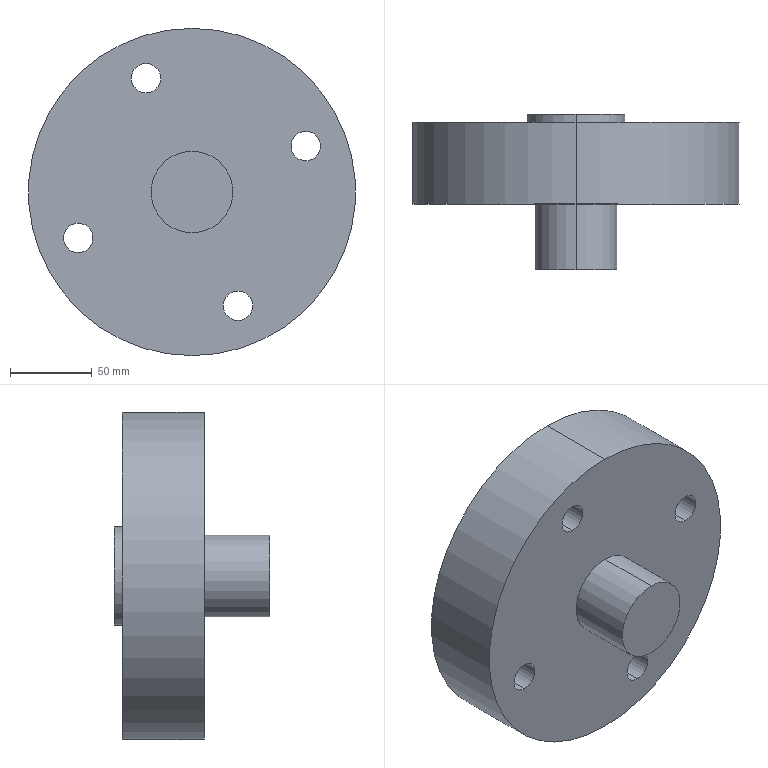Part | SolidWorks | features Chamfer 1, HoleWzd 1, Revolution 1 | 1 solid | 18 faces | box 200 x 95 x 200 mm | volume 1612580 mm3 | cylinder 14 | plane 4 | commonest cylinder face diameters 18 x8 50 x2 60 x2 200 x2
STEP:
#1=CARTESIAN_POINT('',(-69.533,-81.6,-19.109));
#2=VERTEX_POINT('',#1);
#3=CARTESIAN_POINT('',(-69.533,-81.6,-37.109));
#4=VERTEX_POINT('',#3);
#5=CARTESIAN_POINT('',(-69.533,-81.6,-28.109));
#6=DIRECTION('',(0.,-1.,0.));
#7=DIRECTION('',(0.,0.,-1.));
#8=AXIS2_PLACEMENT_3D('',#5,#6,#7);
#9=CIRCLE('',#8,9.);
#10=EDGE_CURVE('',#2,#4,#9,.T.);
#11=ORIENTED_EDGE('',*,*,#10,.T.);
#12=CARTESIAN_POINT('',(-69.533,-31.6,-37.109));
#13=VERTEX_POINT('',#12);
#14=CARTESIAN_POINT('',(-69.533,-31.6,-37.109));
#15=DIRECTION('',(0.,1.,0.));
#16=VECTOR('',#15,1000.);
#17=LINE('',#14,#16);
#18=EDGE_CURVE('',#4,#13,#17,.T.);
#19=ORIENTED_EDGE('',*,*,#18,.T.);
#20=CARTESIAN_POINT('',(-69.533,-31.6,-19.109));
#21=VERTEX_POINT('',#20);
#22=CARTESIAN_POINT('',(-69.533,-31.6,-28.109));
#23=DIRECTION('',(0.,1.,0.));
#24=DIRECTION('',(0.,0.,1.));
#25=AXIS2_PLACEMENT_3D('',#22,#23,#24);
#26=CIRCLE('',#25,9.);
#27=EDGE_CURVE('',#13,#21,#26,.T.);
#28=ORIENTED_EDGE('',*,*,#27,.T.);
#29=CARTESIAN_POINT('',(-69.533,-31.6,-19.109));
#30=DIRECTION('',(0.,1.,0.));
#31=VECTOR('',#30,1000.);
#32=LINE('',#29,#31);
#33=EDGE_CURVE('',#2,#21,#32,.T.);
#34=ORIENTED_EDGE('',*,*,#33,.F.);
#35=EDGE_LOOP('',(#11,#19,#28,#34));
#36=FACE_OUTER_BOUND('',#35,.T.);
#37=CARTESIAN_POINT('',(-69.533,-31.6,-28.109));
#38=DIRECTION('',(0.,1.,0.));
#39=DIRECTION('',(0.,0.,1.));
#40=AXIS2_PLACEMENT_3D('',#37,#38,#39);
#41=CYLINDRICAL_SURFACE('',#40,9.);
#42=ADVANCED_FACE('',(#36),#41,.F.);
#43=CARTESIAN_POINT('',(-28.109,-81.6,78.533));
#44=VERTEX_POINT('',#43);
#45=CARTESIAN_POINT('',(-28.109,-81.6,60.533));
#46=VERTEX_POINT('',#45);
#47=CARTESIAN_POINT('',(-28.109,-81.6,69.533));
#48=DIRECTION('',(0.,-1.,0.));
#49=DIRECTION('',(0.,0.,-1.));
#50=AXIS2_PLACEMENT_3D('',#47,#48,#49);
#51=CIRCLE('',#50,9.);
#52=EDGE_CURVE('',#44,#46,#51,.T.);
#53=ORIENTED_EDGE('',*,*,#52,.T.);
#54=CARTESIAN_POINT('',(-28.109,-31.6,60.533));
#55=VERTEX_POINT('',#54);
#56=CARTESIAN_POINT('',(-28.109,-31.6,60.533));
#57=DIRECTION('',(0.,1.,0.));
#58=VECTOR('',#57,1000.);
#59=LINE('',#56,#58);
#60=EDGE_CURVE('',#46,#55,#59,.T.);
#61=ORIENTED_EDGE('',*,*,#60,.T.);
#62=CARTESIAN_POINT('',(-28.109,-31.6,78.533));
#63=VERTEX_POINT('',#62);
#64=CARTESIAN_POINT('',(-28.109,-31.6,69.533));
#65=DIRECTION('',(0.,1.,0.));
#66=DIRECTION('',(0.,0.,1.));
#67=AXIS2_PLACEMENT_3D('',#64,#65,#66);
#68=CIRCLE('',#67,9.);
#69=EDGE_CURVE('',#55,#63,#68,.T.);
#70=ORIENTED_EDGE('',*,*,#69,.T.);
#71=CARTESIAN_POINT('',(-28.109,-31.6,78.533));
#72=DIRECTION('',(0.,1.,0.));
#73=VECTOR('',#72,1000.);
#74=LINE('',#71,#73);
#75=EDGE_CURVE('',#44,#63,#74,.T.);
#76=ORIENTED_EDGE('',*,*,#75,.F.);
#77=EDGE_LOOP('',(#53,#61,#70,#76));
#78=FACE_OUTER_BOUND('',#77,.T.);
#79=CARTESIAN_POINT('',(-28.109,-31.6,69.533));
#80=DIRECTION('',(0.,1.,0.));
#81=DIRECTION('',(0.,0.,1.));
#82=AXIS2_PLACEMENT_3D('',#79,#80,#81);
#83=CYLINDRICAL_SURFACE('',#82,9.);
#84=ADVANCED_FACE('',(#78),#83,.F.);
#85=CARTESIAN_POINT('',(69.533,-81.6,37.109));
#86=VERTEX_POINT('',#85);
#87=CARTESIAN_POINT('',(69.533,-81.6,19.109));
#88=VERTEX_POINT('',#87);
#89=CARTESIAN_POINT('',(69.533,-81.6,28.109));
#90=DIRECTION('',(0.,-1.,0.));
#91=DIRECTION('',(0.,0.,-1.));
#92=AXIS2_PLACEMENT_3D('',#89,#90,#91);
#93=CIRCLE('',#92,9.);
#94=EDGE_CURVE('',#86,#88,#93,.T.);
#95=ORIENTED_EDGE('',*,*,#94,.T.);
#96=CARTESIAN_POINT('',(69.533,-31.6,19.109));
#97=VERTEX_POINT('',#96);
#98=CARTESIAN_POINT('',(69.533,-31.6,19.109));
#99=DIRECTION('',(0.,1.,0.));
#100=VECTOR('',#99,1000.);
#101=LINE('',#98,#100);
#102=EDGE_CURVE('',#88,#97,#101,.T.);
#103=ORIENTED_EDGE('',*,*,#102,.T.);
#104=CARTESIAN_POINT('',(69.533,-31.6,37.109));
#105=VERTEX_POINT('',#104);
#106=CARTESIAN_POINT('',(69.533,-31.6,28.109));
#107=DIRECTION('',(0.,1.,0.));
#108=DIRECTION('',(0.,0.,1.));
#109=AXIS2_PLACEMENT_3D('',#106,#107,#108);
#110=CIRCLE('',#109,9.);
#111=EDGE_CURVE('',#97,#105,#110,.T.);
#112=ORIENTED_EDGE('',*,*,#111,.T.);
#113=CARTESIAN_POINT('',(69.533,-31.6,37.109));
#114=DIRECTION('',(0.,1.,0.));
#115=VECTOR('',#114,1000.);
#116=LINE('',#113,#115);
#117=EDGE_CURVE('',#86,#105,#116,.T.);
#118=ORIENTED_EDGE('',*,*,#117,.F.);
#119=EDGE_LOOP('',(#95,#103,#112,#118));
#120=FACE_OUTER_BOUND('',#119,.T.);
#121=CARTESIAN_POINT('',(69.533,-31.6,28.109));
#122=DIRECTION('',(0.,1.,0.));
#123=DIRECTION('',(0.,0.,1.));
#124=AXIS2_PLACEMENT_3D('',#121,#122,#123);
#125=CYLINDRICAL_SURFACE('',#124,9.);
#126=ADVANCED_FACE('',(#120),#125,.F.);
#127=CARTESIAN_POINT('',(28.109,-81.6,-60.533));
#128=VERTEX_POINT('',#127);
#129=CARTESIAN_POINT('',(28.109,-81.6,-78.533));
#130=VERTEX_POINT('',#129);
#131=CARTESIAN_POINT('',(28.109,-81.6,-69.533));
#132=DIRECTION('',(0.,-1.,0.));
#133=DIRECTION('',(0.,0.,-1.));
#134=AXIS2_PLACEMENT_3D('',#131,#132,#133);
#135=CIRCLE('',#134,9.);
#136=EDGE_CURVE('',#128,#130,#135,.T.);
#137=ORIENTED_EDGE('',*,*,#136,.T.);
#138=CARTESIAN_POINT('',(28.109,-31.6,-78.533));
#139=VERTEX_POINT('',#138);
#140=CARTESIAN_POINT('',(28.109,-31.6,-78.533));
#141=DIRECTION('',(0.,1.,0.));
#142=VECTOR('',#141,1000.);
#143=LINE('',#140,#142);
#144=EDGE_CURVE('',#130,#139,#143,.T.);
#145=ORIENTED_EDGE('',*,*,#144,.T.);
#146=CARTESIAN_POINT('',(28.109,-31.6,-60.533));
#147=VERTEX_POINT('',#146);
#148=CARTESIAN_POINT('',(28.109,-31.6,-69.533));
#149=DIRECTION('',(0.,1.,0.));
#150=DIRECTION('',(0.,0.,1.));
#151=AXIS2_PLACEMENT_3D('',#148,#149,#150);
#152=CIRCLE('',#151,9.);
#153=EDGE_CURVE('',#139,#147,#152,.T.);
#154=ORIENTED_EDGE('',*,*,#153,.T.);
#155=CARTESIAN_POINT('',(28.109,-31.6,-60.533));
#156=DIRECTION('',(0.,1.,0.));
#157=VECTOR('',#156,1000.);
#158=LINE('',#155,#157);
#159=EDGE_CURVE('',#128,#147,#158,.T.);
#160=ORIENTED_EDGE('',*,*,#159,.F.);
#161=EDGE_LOOP('',(#137,#145,#154,#160));
#162=FACE_OUTER_BOUND('',#161,.T.);
#163=CARTESIAN_POINT('',(28.109,-31.6,-69.533));
#164=DIRECTION('',(0.,1.,0.));
#165=DIRECTION('',(0.,0.,1.));
#166=AXIS2_PLACEMENT_3D('',#163,#164,#165);
#167=CYLINDRICAL_SURFACE('',#166,9.);
#168=ADVANCED_FACE('',(#162),#167,.F.);
#169=CARTESIAN_POINT('',(0.,-26.6,-30.));
#170=VERTEX_POINT('',#169);
#171=CARTESIAN_POINT('',(0.,-26.6,30.));
#172=VERTEX_POINT('',#171);
#173=CARTESIAN_POINT('',(0.,-26.6,0.));
#174=DIRECTION('',(0.,-1.,0.));
#175=DIRECTION('',(0.,0.,-1.));
#176=AXIS2_PLACEMENT_3D('',#173,#174,#175);
#177=CIRCLE('',#176,30.);
#178=EDGE_CURVE('',#170,#172,#177,.T.);
#179=ORIENTED_EDGE('',*,*,#178,.T.);
#180=CARTESIAN_POINT('',(0.,-31.6,30.));
#181=VERTEX_POINT('',#180);
#182=CARTESIAN_POINT('',(0.,0.,30.));
#183=DIRECTION('',(0.,-1.,0.));
#184=VECTOR('',#183,1000.);
#185=LINE('',#182,#184);
#186=EDGE_CURVE('',#172,#181,#185,.T.);
#187=ORIENTED_EDGE('',*,*,#186,.T.);
#188=CARTESIAN_POINT('',(0.,-31.6,-30.));
#189=VERTEX_POINT('',#188);
#190=CARTESIAN_POINT('',(0.,-31.6,0.));
#191=DIRECTION('',(0.,-1.,0.));
#192=DIRECTION('',(0.,0.,-1.));
#193=AXIS2_PLACEMENT_3D('',#190,#191,#192);
#194=CIRCLE('',#193,30.);
#195=EDGE_CURVE('',#189,#181,#194,.T.);
#196=ORIENTED_EDGE('',*,*,#195,.F.);
#197=CARTESIAN_POINT('',(0.,0.,-30.));
#198=DIRECTION('',(0.,-1.,0.));
#199=VECTOR('',#198,1000.);
#200=LINE('',#197,#199);
#201=EDGE_CURVE('',#170,#189,#200,.T.);
#202=ORIENTED_EDGE('',*,*,#201,.F.);
#203=EDGE_LOOP('',(#179,#187,#196,#202));
#204=FACE_OUTER_BOUND('',#203,.T.);
#205=CARTESIAN_POINT('',(0.,0.,0.));
#206=DIRECTION('',(0.,-1.,0.));
#207=DIRECTION('',(0.,0.,-1.));
#208=AXIS2_PLACEMENT_3D('',#205,#206,#207);
#209=CYLINDRICAL_SURFACE('',#208,30.);
#210=ADVANCED_FACE('',(#204),#209,.T.);
#211=CARTESIAN_POINT('',(0.,-31.6,-100.));
#212=VERTEX_POINT('',#211);
#213=CARTESIAN_POINT('',(0.,-31.6,100.));
#214=VERTEX_POINT('',#213);
#215=CARTESIAN_POINT('',(0.,-31.6,0.));
#216=DIRECTION('',(0.,-1.,0.));
#217=DIRECTION('',(0.,0.,-1.));
#218=AXIS2_PLACEMENT_3D('',#215,#216,#217);
#219=CIRCLE('',#218,100.);
#220=EDGE_CURVE('',#212,#214,#219,.T.);
#221=ORIENTED_EDGE('',*,*,#220,.T.);
#222=CARTESIAN_POINT('',(0.,-81.6,100.));
#223=VERTEX_POINT('',#222);
#224=CARTESIAN_POINT('',(0.,0.,100.));
#225=DIRECTION('',(0.,-1.,0.));
#226=VECTOR('',#225,1000.);
#227=LINE('',#224,#226);
#228=EDGE_CURVE('',#214,#223,#227,.T.);
#229=ORIENTED_EDGE('',*,*,#228,.T.);
#230=CARTESIAN_POINT('',(0.,-81.6,-100.));
#231=VERTEX_POINT('',#230);
#232=CARTESIAN_POINT('',(0.,-81.6,0.));
#233=DIRECTION('',(0.,-1.,0.));
#234=DIRECTION('',(0.,0.,-1.));
#235=AXIS2_PLACEMENT_3D('',#232,#233,#234);
#236=CIRCLE('',#235,100.);
#237=EDGE_CURVE('',#231,#223,#236,.T.);
#238=ORIENTED_EDGE('',*,*,#237,.F.);
#239=CARTESIAN_POINT('',(0.,0.,-100.));
#240=DIRECTION('',(0.,-1.,0.));
#241=VECTOR('',#240,1000.);
#242=LINE('',#239,#241);
#243=EDGE_CURVE('',#212,#231,#242,.T.);
#244=ORIENTED_EDGE('',*,*,#243,.F.);
#245=EDGE_LOOP('',(#221,#229,#238,#244));
#246=FACE_OUTER_BOUND('',#245,.T.);
#247=CARTESIAN_POINT('',(0.,0.,0.));
#248=DIRECTION('',(0.,-1.,0.));
#249=DIRECTION('',(0.,0.,-1.));
#250=AXIS2_PLACEMENT_3D('',#247,#248,#249);
#251=CYLINDRICAL_SURFACE('',#250,100.);
#252=ADVANCED_FACE('',(#246),#251,.T.);
#253=CARTESIAN_POINT('',(0.,-81.6,-25.));
#254=VERTEX_POINT('',#253);
#255=CARTESIAN_POINT('',(0.,-81.6,25.));
#256=VERTEX_POINT('',#255);
#257=CARTESIAN_POINT('',(0.,-81.6,0.));
#258=DIRECTION('',(0.,-1.,0.));
#259=DIRECTION('',(0.,0.,-1.));
#260=AXIS2_PLACEMENT_3D('',#257,#258,#259);
#261=CIRCLE('',#260,25.);
#262=EDGE_CURVE('',#254,#256,#261,.T.);
#263=ORIENTED_EDGE('',*,*,#262,.T.);
#264=CARTESIAN_POINT('',(0.,-121.6,25.));
#265=VERTEX_POINT('',#264);
#266=CARTESIAN_POINT('',(0.,0.,25.));
#267=DIRECTION('',(0.,-1.,0.));
#268=VECTOR('',#267,1000.);
#269=LINE('',#266,#268);
#270=EDGE_CURVE('',#256,#265,#269,.T.);
#271=ORIENTED_EDGE('',*,*,#270,.T.);
#272=CARTESIAN_POINT('',(0.,-121.6,-25.));
#273=VERTEX_POINT('',#272);
#274=CARTESIAN_POINT('',(0.,-121.6,0.));
#275=DIRECTION('',(0.,-1.,0.));
#276=DIRECTION('',(0.,0.,-1.));
#277=AXIS2_PLACEMENT_3D('',#274,#275,#276);
#278=CIRCLE('',#277,25.);
#279=EDGE_CURVE('',#273,#265,#278,.T.);
#280=ORIENTED_EDGE('',*,*,#279,.F.);
#281=CARTESIAN_POINT('',(0.,0.,-25.));
#282=DIRECTION('',(0.,-1.,0.));
#283=VECTOR('',#282,1000.);
#284=LINE('',#281,#283);
#285=EDGE_CURVE('',#254,#273,#284,.T.);
#286=ORIENTED_EDGE('',*,*,#285,.F.);
#287=EDGE_LOOP('',(#263,#271,#280,#286));
#288=FACE_OUTER_BOUND('',#287,.T.);
#289=CARTESIAN_POINT('',(0.,0.,0.));
#290=DIRECTION('',(0.,-1.,0.));
#291=DIRECTION('',(0.,0.,-1.));
#292=AXIS2_PLACEMENT_3D('',#289,#290,#291);
#293=CYLINDRICAL_SURFACE('',#292,25.);
#294=ADVANCED_FACE('',(#288),#293,.T.);
#295=ORIENTED_EDGE('',*,*,#279,.T.);
#296=CARTESIAN_POINT('',(0.,-121.6,0.));
#297=DIRECTION('',(0.,-1.,0.));
#298=DIRECTION('',(0.,0.,-1.));
#299=AXIS2_PLACEMENT_3D('',#296,#297,#298);
#300=CIRCLE('',#299,25.);
#301=EDGE_CURVE('',#265,#273,#300,.T.);
#302=ORIENTED_EDGE('',*,*,#301,.T.);
#303=EDGE_LOOP('',(#295,#302));
#304=FACE_OUTER_BOUND('',#303,.T.);
#305=CARTESIAN_POINT('',(25.,-121.6,0.));
#306=DIRECTION('',(0.,-1.,0.));
#307=DIRECTION('',(0.,0.,-1.));
#308=AXIS2_PLACEMENT_3D('',#305,#306,#307);
#309=PLANE('',#308);
#310=ADVANCED_FACE('',(#304),#309,.T.);
#311=ORIENTED_EDGE('',*,*,#270,.F.);
#312=CARTESIAN_POINT('',(0.,-81.6,0.));
#313=DIRECTION('',(0.,-1.,0.));
#314=DIRECTION('',(0.,0.,-1.));
#315=AXIS2_PLACEMENT_3D('',#312,#313,#314);
#316=CIRCLE('',#315,25.);
#317=EDGE_CURVE('',#256,#254,#316,.T.);
#318=ORIENTED_EDGE('',*,*,#317,.T.);
#319=ORIENTED_EDGE('',*,*,#285,.T.);
#320=ORIENTED_EDGE('',*,*,#301,.F.);
#321=EDGE_LOOP('',(#311,#318,#319,#320));
#322=FACE_OUTER_BOUND('',#321,.T.);
#323=CARTESIAN_POINT('',(0.,0.,0.));
#324=DIRECTION('',(0.,-1.,0.));
#325=DIRECTION('',(0.,0.,-1.));
#326=AXIS2_PLACEMENT_3D('',#323,#324,#325);
#327=CYLINDRICAL_SURFACE('',#326,25.);
#328=ADVANCED_FACE('',(#322),#327,.T.);
#329=ORIENTED_EDGE('',*,*,#10,.F.);
#330=CARTESIAN_POINT('',(-69.533,-81.6,-28.109));
#331=DIRECTION('',(0.,-1.,0.));
#332=DIRECTION('',(0.,0.,-1.));
#333=AXIS2_PLACEMENT_3D('',#330,#331,#332);
#334=CIRCLE('',#333,9.);
#335=EDGE_CURVE('',#4,#2,#334,.T.);
#336=ORIENTED_EDGE('',*,*,#335,.F.);
#337=EDGE_LOOP('',(#329,#336));
#338=FACE_BOUND('',#337,.T.);
#339=ORIENTED_EDGE('',*,*,#52,.F.);
#340=CARTESIAN_POINT('',(-28.109,-81.6,69.533));
#341=DIRECTION('',(0.,-1.,0.));
#342=DIRECTION('',(0.,0.,-1.));
#343=AXIS2_PLACEMENT_3D('',#340,#341,#342);
#344=CIRCLE('',#343,9.);
#345=EDGE_CURVE('',#46,#44,#344,.T.);
#346=ORIENTED_EDGE('',*,*,#345,.F.);
#347=EDGE_LOOP('',(#339,#346));
#348=FACE_BOUND('',#347,.T.);
#349=ORIENTED_EDGE('',*,*,#94,.F.);
#350=CARTESIAN_POINT('',(69.533,-81.6,28.109));
#351=DIRECTION('',(0.,-1.,0.));
#352=DIRECTION('',(0.,0.,-1.));
#353=AXIS2_PLACEMENT_3D('',#350,#351,#352);
#354=CIRCLE('',#353,9.);
#355=EDGE_CURVE('',#88,#86,#354,.T.);
#356=ORIENTED_EDGE('',*,*,#355,.F.);
#357=EDGE_LOOP('',(#349,#356));
#358=FACE_BOUND('',#357,.T.);
#359=ORIENTED_EDGE('',*,*,#136,.F.);
#360=CARTESIAN_POINT('',(28.109,-81.6,-69.533));
#361=DIRECTION('',(0.,-1.,0.));
#362=DIRECTION('',(0.,0.,-1.));
#363=AXIS2_PLACEMENT_3D('',#360,#361,#362);
#364=CIRCLE('',#363,9.);
#365=EDGE_CURVE('',#130,#128,#364,.T.);
#366=ORIENTED_EDGE('',*,*,#365,.F.);
#367=EDGE_LOOP('',(#359,#366));
#368=FACE_BOUND('',#367,.T.);
#369=ORIENTED_EDGE('',*,*,#237,.T.);
#370=CARTESIAN_POINT('',(0.,-81.6,0.));
#371=DIRECTION('',(0.,-1.,0.));
#372=DIRECTION('',(0.,0.,-1.));
#373=AXIS2_PLACEMENT_3D('',#370,#371,#372);
#374=CIRCLE('',#373,100.);
#375=EDGE_CURVE('',#223,#231,#374,.T.);
#376=ORIENTED_EDGE('',*,*,#375,.T.);
#377=EDGE_LOOP('',(#369,#376));
#378=FACE_OUTER_BOUND('',#377,.T.);
#379=ORIENTED_EDGE('',*,*,#262,.F.);
#380=ORIENTED_EDGE('',*,*,#317,.F.);
#381=EDGE_LOOP('',(#379,#380));
#382=FACE_BOUND('',#381,.T.);
#383=CARTESIAN_POINT('',(100.,-81.6,0.));
#384=DIRECTION('',(0.,-1.,0.));
#385=DIRECTION('',(0.,0.,-1.));
#386=AXIS2_PLACEMENT_3D('',#383,#384,#385);
#387=PLANE('',#386);
#388=ADVANCED_FACE('',(#338,#348,#358,#368,#378,#382),#387,.T.);
#389=ORIENTED_EDGE('',*,*,#228,.F.);
#390=CARTESIAN_POINT('',(0.,-31.6,0.));
#391=DIRECTION('',(0.,-1.,0.));
#392=DIRECTION('',(0.,0.,-1.));
#393=AXIS2_PLACEMENT_3D('',#390,#391,#392);
#394=CIRCLE('',#393,100.);
#395=EDGE_CURVE('',#214,#212,#394,.T.);
#396=ORIENTED_EDGE('',*,*,#395,.T.);
#397=ORIENTED_EDGE('',*,*,#243,.T.);
#398=ORIENTED_EDGE('',*,*,#375,.F.);
#399=EDGE_LOOP('',(#389,#396,#397,#398));
#400=FACE_OUTER_BOUND('',#399,.T.);
#401=CARTESIAN_POINT('',(0.,0.,0.));
#402=DIRECTION('',(0.,-1.,0.));
#403=DIRECTION('',(0.,0.,-1.));
#404=AXIS2_PLACEMENT_3D('',#401,#402,#403);
#405=CYLINDRICAL_SURFACE('',#404,100.);
#406=ADVANCED_FACE('',(#400),#405,.T.);
#407=CARTESIAN_POINT('',(-69.533,-31.6,-28.109));
#408=DIRECTION('',(0.,1.,0.));
#409=DIRECTION('',(0.,0.,1.));
#410=AXIS2_PLACEMENT_3D('',#407,#408,#409);
#411=CIRCLE('',#410,9.);
#412=EDGE_CURVE('',#21,#13,#411,.T.);
#413=ORIENTED_EDGE('',*,*,#412,.F.);
#414=ORIENTED_EDGE('',*,*,#27,.F.);
#415=EDGE_LOOP('',(#413,#414));
#416=FACE_BOUND('',#415,.T.);
#417=CARTESIAN_POINT('',(-28.109,-31.6,69.533));
#418=DIRECTION('',(0.,1.,0.));
#419=DIRECTION('',(0.,0.,1.));
#420=AXIS2_PLACEMENT_3D('',#417,#418,#419);
#421=CIRCLE('',#420,9.);
#422=EDGE_CURVE('',#63,#55,#421,.T.);
#423=ORIENTED_EDGE('',*,*,#422,.F.);
#424=ORIENTED_EDGE('',*,*,#69,.F.);
#425=EDGE_LOOP('',(#423,#424));
#426=FACE_BOUND('',#425,.T.);
#427=CARTESIAN_POINT('',(69.533,-31.6,28.109));
#428=DIRECTION('',(0.,1.,0.));
#429=DIRECTION('',(0.,0.,1.));
#430=AXIS2_PLACEMENT_3D('',#427,#428,#429);
#431=CIRCLE('',#430,9.);
#432=EDGE_CURVE('',#105,#97,#431,.T.);
#433=ORIENTED_EDGE('',*,*,#432,.F.);
#434=ORIENTED_EDGE('',*,*,#111,.F.);
#435=EDGE_LOOP('',(#433,#434));
#436=FACE_BOUND('',#435,.T.);
#437=CARTESIAN_POINT('',(28.109,-31.6,-69.533));
#438=DIRECTION('',(0.,1.,0.));
#439=DIRECTION('',(0.,0.,1.));
#440=AXIS2_PLACEMENT_3D('',#437,#438,#439);
#441=CIRCLE('',#440,9.);
#442=EDGE_CURVE('',#147,#139,#441,.T.);
#443=ORIENTED_EDGE('',*,*,#442,.F.);
#444=ORIENTED_EDGE('',*,*,#153,.F.);
#445=EDGE_LOOP('',(#443,#444));
#446=FACE_BOUND('',#445,.T.);
#447=ORIENTED_EDGE('',*,*,#195,.T.);
#448=CARTESIAN_POINT('',(0.,-31.6,0.));
#449=DIRECTION('',(0.,-1.,0.));
#450=DIRECTION('',(0.,0.,-1.));
#451=AXIS2_PLACEMENT_3D('',#448,#449,#450);
#452=CIRCLE('',#451,30.);
#453=EDGE_CURVE('',#181,#189,#452,.T.);
#454=ORIENTED_EDGE('',*,*,#453,.T.);
#455=EDGE_LOOP('',(#447,#454));
#456=FACE_BOUND('',#455,.T.);
#457=ORIENTED_EDGE('',*,*,#220,.F.);
#458=ORIENTED_EDGE('',*,*,#395,.F.);
#459=EDGE_LOOP('',(#457,#458));
#460=FACE_OUTER_BOUND('',#459,.T.);
#461=CARTESIAN_POINT('',(30.,-31.6,0.));
#462=DIRECTION('',(0.,1.,0.));
#463=DIRECTION('',(0.,0.,1.));
#464=AXIS2_PLACEMENT_3D('',#461,#462,#463);
#465=PLANE('',#464);
#466=ADVANCED_FACE('',(#416,#426,#436,#446,#456,#460),#465,.T.);
#467=ORIENTED_EDGE('',*,*,#186,.F.);
#468=CARTESIAN_POINT('',(0.,-26.6,0.));
#469=DIRECTION('',(0.,-1.,0.));
#470=DIRECTION('',(0.,0.,-1.));
#471=AXIS2_PLACEMENT_3D('',#468,#469,#470);
#472=CIRCLE('',#471,30.);
#473=EDGE_CURVE('',#172,#170,#472,.T.);
#474=ORIENTED_EDGE('',*,*,#473,.T.);
#475=ORIENTED_EDGE('',*,*,#201,.T.);
#476=ORIENTED_EDGE('',*,*,#453,.F.);
#477=EDGE_LOOP('',(#467,#474,#475,#476));
#478=FACE_OUTER_BOUND('',#477,.T.);
#479=CARTESIAN_POINT('',(0.,0.,0.));
#480=DIRECTION('',(0.,-1.,0.));
#481=DIRECTION('',(0.,0.,-1.));
#482=AXIS2_PLACEMENT_3D('',#479,#480,#481);
#483=CYLINDRICAL_SURFACE('',#482,30.);
#484=ADVANCED_FACE('',(#478),#483,.T.);
#485=ORIENTED_EDGE('',*,*,#178,.F.);
#486=ORIENTED_EDGE('',*,*,#473,.F.);
#487=EDGE_LOOP('',(#485,#486));
#488=FACE_OUTER_BOUND('',#487,.T.);
#489=CARTESIAN_POINT('',(30.,-26.6,0.));
#490=DIRECTION('',(0.,1.,0.));
#491=DIRECTION('',(0.,0.,1.));
#492=AXIS2_PLACEMENT_3D('',#489,#490,#491);
#493=PLANE('',#492);
#494=ADVANCED_FACE('',(#488),#493,.T.);
#495=ORIENTED_EDGE('',*,*,#144,.F.);
#496=ORIENTED_EDGE('',*,*,#365,.T.);
#497=ORIENTED_EDGE('',*,*,#159,.T.);
#498=ORIENTED_EDGE('',*,*,#442,.T.);
#499=EDGE_LOOP('',(#495,#496,#497,#498));
#500=FACE_OUTER_BOUND('',#499,.T.);
#501=CARTESIAN_POINT('',(28.109,-31.6,-69.533));
#502=DIRECTION('',(0.,1.,0.));
#503=DIRECTION('',(0.,0.,1.));
#504=AXIS2_PLACEMENT_3D('',#501,#502,#503);
#505=CYLINDRICAL_SURFACE('',#504,9.);
#506=ADVANCED_FACE('',(#500),#505,.F.);
#507=ORIENTED_EDGE('',*,*,#102,.F.);
#508=ORIENTED_EDGE('',*,*,#355,.T.);
#509=ORIENTED_EDGE('',*,*,#117,.T.);
#510=ORIENTED_EDGE('',*,*,#432,.T.);
#511=EDGE_LOOP('',(#507,#508,#509,#510));
#512=FACE_OUTER_BOUND('',#511,.T.);
#513=CARTESIAN_POINT('',(69.533,-31.6,28.109));
#514=DIRECTION('',(0.,1.,0.));
#515=DIRECTION('',(0.,0.,1.));
#516=AXIS2_PLACEMENT_3D('',#513,#514,#515);
#517=CYLINDRICAL_SURFACE('',#516,9.);
#518=ADVANCED_FACE('',(#512),#517,.F.);
#519=ORIENTED_EDGE('',*,*,#60,.F.);
#520=ORIENTED_EDGE('',*,*,#345,.T.);
#521=ORIENTED_EDGE('',*,*,#75,.T.);
#522=ORIENTED_EDGE('',*,*,#422,.T.);
#523=EDGE_LOOP('',(#519,#520,#521,#522));
#524=FACE_OUTER_BOUND('',#523,.T.);
#525=CARTESIAN_POINT('',(-28.109,-31.6,69.533));
#526=DIRECTION('',(0.,1.,0.));
#527=DIRECTION('',(0.,0.,1.));
#528=AXIS2_PLACEMENT_3D('',#525,#526,#527);
#529=CYLINDRICAL_SURFACE('',#528,9.);
#530=ADVANCED_FACE('',(#524),#529,.F.);
#531=ORIENTED_EDGE('',*,*,#18,.F.);
#532=ORIENTED_EDGE('',*,*,#335,.T.);
#533=ORIENTED_EDGE('',*,*,#33,.T.);
#534=ORIENTED_EDGE('',*,*,#412,.T.);
#535=EDGE_LOOP('',(#531,#532,#533,#534));
#536=FACE_OUTER_BOUND('',#535,.T.);
#537=CARTESIAN_POINT('',(-69.533,-31.6,-28.109));
#538=DIRECTION('',(0.,1.,0.));
#539=DIRECTION('',(0.,0.,1.));
#540=AXIS2_PLACEMENT_3D('',#537,#538,#539);
#541=CYLINDRICAL_SURFACE('',#540,9.);
#542=ADVANCED_FACE('',(#536),#541,.F.);
#543=CLOSED_SHELL('',(#42,#84,#126,#168,#210,#252,#294,#310,#328,#388,#406,#466,#484,#494,#506,#518,#530,#542));
#544=MANIFOLD_SOLID_BREP('',#543);
#545=CARTESIAN_POINT('',(0.,0.,0.));
#546=DIRECTION('',(0.,0.,1.));
#547=DIRECTION('',(1.,0.,0.));
#548=AXIS2_PLACEMENT_3D('',#545,#546,#547);
#549=(LENGTH_UNIT()NAMED_UNIT(*)SI_UNIT(.MILLI.,.METRE.));
#550=UNCERTAINTY_MEASURE_WITH_UNIT(LENGTH_MEASURE(0.00001),#549,'','');
#551=(NAMED_UNIT(*)PLANE_ANGLE_UNIT()SI_UNIT($,.RADIAN.));
#552=(NAMED_UNIT(*)SI_UNIT($,.STERADIAN.)SOLID_ANGLE_UNIT());
#553=(GEOMETRIC_REPRESENTATION_CONTEXT(3)GLOBAL_UNCERTAINTY_ASSIGNED_CONTEXT((#550))GLOBAL_UNIT_ASSIGNED_CONTEXT((#549,#551,#552))REPRESENTATION_CONTEXT('',''));
#554=ADVANCED_BREP_SHAPE_REPRESENTATION('',(#544,#548),#553);